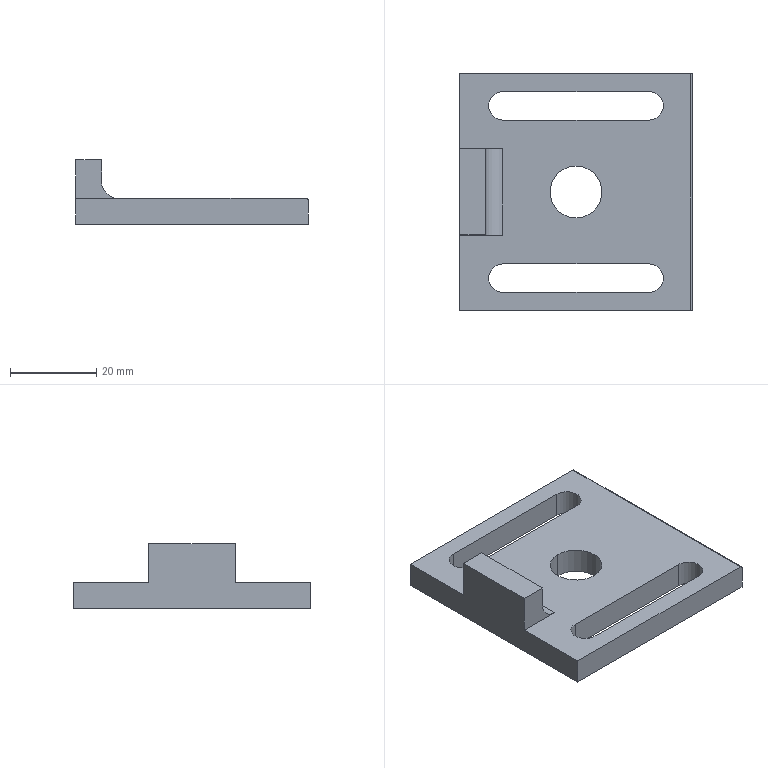Part | STEP file | TNSN20-Y20-F22-Part-4 | 1 solid | 22 faces | box 54 x 55 x 15 mm | volume 15184 mm3 | plane 14 | cylinder 8 | commonest cylinder face diameters 6.6 x4 12 x2 1 x1 8 x1
STEP:
#1=CARTESIAN_POINT('',(14056.745,13710.046,24.));
#2=VERTEX_POINT('',#1);
#3=CARTESIAN_POINT('',(14056.745,13730.046,24.));
#4=VERTEX_POINT('',#3);
#5=CARTESIAN_POINT('',(14056.745,13710.046,24.));
#6=DIRECTION('',(0.,1.,0.));
#7=VECTOR('',#6,1000.);
#8=LINE('',#5,#7);
#9=EDGE_CURVE('',#2,#4,#8,.T.);
#10=ORIENTED_EDGE('',*,*,#9,.T.);
#11=CARTESIAN_POINT('',(14050.745,13730.046,24.));
#12=VERTEX_POINT('',#11);
#13=CARTESIAN_POINT('',(14056.745,13730.046,24.));
#14=DIRECTION('',(-1.,0.,0.));
#15=VECTOR('',#14,1000.);
#16=LINE('',#13,#15);
#17=EDGE_CURVE('',#4,#12,#16,.T.);
#18=ORIENTED_EDGE('',*,*,#17,.T.);
#19=CARTESIAN_POINT('',(14050.745,13710.046,24.));
#20=VERTEX_POINT('',#19);
#21=CARTESIAN_POINT('',(14050.745,13710.046,24.));
#22=DIRECTION('',(0.,1.,0.));
#23=VECTOR('',#22,1000.);
#24=LINE('',#21,#23);
#25=EDGE_CURVE('',#20,#12,#24,.T.);
#26=ORIENTED_EDGE('',*,*,#25,.F.);
#27=CARTESIAN_POINT('',(14050.745,13710.046,24.));
#28=DIRECTION('',(1.,0.,0.));
#29=VECTOR('',#28,1000.);
#30=LINE('',#27,#29);
#31=EDGE_CURVE('',#20,#2,#30,.T.);
#32=ORIENTED_EDGE('',*,*,#31,.T.);
#33=EDGE_LOOP('',(#10,#18,#26,#32));
#34=FACE_OUTER_BOUND('',#33,.T.);
#35=CARTESIAN_POINT('',(14038.084,13704.386,24.));
#36=DIRECTION('',(0.,0.,-1.));
#37=DIRECTION('',(0.,1.,0.));
#38=AXIS2_PLACEMENT_3D('',#35,#36,#37);
#39=PLANE('',#38);
#40=ADVANCED_FACE('',(#34),#39,.F.);
#41=ORIENTED_EDGE('',*,*,#25,.T.);
#42=CARTESIAN_POINT('',(14050.745,13730.046,15.));
#43=VERTEX_POINT('',#42);
#44=CARTESIAN_POINT('',(14050.745,13730.046,24.));
#45=DIRECTION('',(0.,0.,-1.));
#46=VECTOR('',#45,1000.);
#47=LINE('',#44,#46);
#48=EDGE_CURVE('',#12,#43,#47,.T.);
#49=ORIENTED_EDGE('',*,*,#48,.T.);
#50=CARTESIAN_POINT('',(14050.745,13747.546,15.));
#51=VERTEX_POINT('',#50);
#52=CARTESIAN_POINT('',(14050.745,13730.046,15.));
#53=DIRECTION('',(0.,1.,0.));
#54=VECTOR('',#53,1000.);
#55=LINE('',#52,#54);
#56=EDGE_CURVE('',#43,#51,#55,.T.);
#57=ORIENTED_EDGE('',*,*,#56,.T.);
#58=CARTESIAN_POINT('',(14050.745,13747.546,9.));
#59=VERTEX_POINT('',#58);
#60=CARTESIAN_POINT('',(14050.745,13747.546,15.));
#61=DIRECTION('',(0.,0.,-1.));
#62=VECTOR('',#61,1000.);
#63=LINE('',#60,#62);
#64=EDGE_CURVE('',#51,#59,#63,.T.);
#65=ORIENTED_EDGE('',*,*,#64,.T.);
#66=CARTESIAN_POINT('',(14050.745,13692.546,9.));
#67=VERTEX_POINT('',#66);
#68=CARTESIAN_POINT('',(14050.745,13692.546,9.));
#69=DIRECTION('',(0.,1.,0.));
#70=VECTOR('',#69,1000.);
#71=LINE('',#68,#70);
#72=EDGE_CURVE('',#67,#59,#71,.T.);
#73=ORIENTED_EDGE('',*,*,#72,.F.);
#74=CARTESIAN_POINT('',(14050.745,13692.546,15.));
#75=VERTEX_POINT('',#74);
#76=CARTESIAN_POINT('',(14050.745,13692.546,15.));
#77=DIRECTION('',(0.,0.,-1.));
#78=VECTOR('',#77,1000.);
#79=LINE('',#76,#78);
#80=EDGE_CURVE('',#75,#67,#79,.T.);
#81=ORIENTED_EDGE('',*,*,#80,.F.);
#82=CARTESIAN_POINT('',(14050.745,13710.046,15.));
#83=VERTEX_POINT('',#82);
#84=CARTESIAN_POINT('',(14050.745,13692.546,15.));
#85=DIRECTION('',(0.,1.,0.));
#86=VECTOR('',#85,1000.);
#87=LINE('',#84,#86);
#88=EDGE_CURVE('',#75,#83,#87,.T.);
#89=ORIENTED_EDGE('',*,*,#88,.T.);
#90=CARTESIAN_POINT('',(14050.745,13710.046,15.));
#91=DIRECTION('',(0.,0.,1.));
#92=VECTOR('',#91,1000.);
#93=LINE('',#90,#92);
#94=EDGE_CURVE('',#83,#20,#93,.T.);
#95=ORIENTED_EDGE('',*,*,#94,.T.);
#96=EDGE_LOOP('',(#41,#49,#57,#65,#73,#81,#89,#95));
#97=FACE_OUTER_BOUND('',#96,.T.);
#98=CARTESIAN_POINT('',(14050.745,13677.29,-26.257));
#99=DIRECTION('',(1.,0.,0.));
#100=DIRECTION('',(0.,1.,0.));
#101=AXIS2_PLACEMENT_3D('',#98,#99,#100);
#102=PLANE('',#101);
#103=ADVANCED_FACE('',(#97),#102,.F.);
#104=CARTESIAN_POINT('',(14104.745,13747.546,9.));
#105=VERTEX_POINT('',#104);
#106=CARTESIAN_POINT('',(14050.745,13747.546,9.));
#107=DIRECTION('',(1.,0.,0.));
#108=VECTOR('',#107,1000.);
#109=LINE('',#106,#108);
#110=EDGE_CURVE('',#59,#105,#109,.T.);
#111=ORIENTED_EDGE('',*,*,#110,.T.);
#112=CARTESIAN_POINT('',(14104.745,13692.546,9.));
#113=VERTEX_POINT('',#112);
#114=CARTESIAN_POINT('',(14104.745,13692.546,9.));
#115=DIRECTION('',(0.,1.,0.));
#116=VECTOR('',#115,1000.);
#117=LINE('',#114,#116);
#118=EDGE_CURVE('',#113,#105,#117,.T.);
#119=ORIENTED_EDGE('',*,*,#118,.F.);
#120=CARTESIAN_POINT('',(14050.745,13692.546,9.));
#121=DIRECTION('',(1.,0.,0.));
#122=VECTOR('',#121,1000.);
#123=LINE('',#120,#122);
#124=EDGE_CURVE('',#67,#113,#123,.T.);
#125=ORIENTED_EDGE('',*,*,#124,.F.);
#126=ORIENTED_EDGE('',*,*,#72,.T.);
#127=EDGE_LOOP('',(#111,#119,#125,#126));
#128=FACE_OUTER_BOUND('',#127,.T.);
#129=CARTESIAN_POINT('',(14094.745,13703.346,9.));
#130=VERTEX_POINT('',#129);
#131=CARTESIAN_POINT('',(14060.745,13703.346,9.));
#132=VERTEX_POINT('',#131);
#133=CARTESIAN_POINT('',(14094.745,13703.346,9.));
#134=DIRECTION('',(-1.,0.,0.));
#135=VECTOR('',#134,1000.);
#136=LINE('',#133,#135);
#137=EDGE_CURVE('',#130,#132,#136,.T.);
#138=ORIENTED_EDGE('',*,*,#137,.T.);
#139=CARTESIAN_POINT('',(14060.745,13696.746,9.));
#140=VERTEX_POINT('',#139);
#141=CARTESIAN_POINT('',(14060.745,13700.046,9.));
#142=DIRECTION('',(0.,0.,1.));
#143=DIRECTION('',(0.,1.,0.));
#144=AXIS2_PLACEMENT_3D('',#141,#142,#143);
#145=CIRCLE('',#144,3.3);
#146=EDGE_CURVE('',#132,#140,#145,.T.);
#147=ORIENTED_EDGE('',*,*,#146,.T.);
#148=CARTESIAN_POINT('',(14094.745,13696.746,9.));
#149=VERTEX_POINT('',#148);
#150=CARTESIAN_POINT('',(14060.745,13696.746,9.));
#151=DIRECTION('',(1.,0.,0.));
#152=VECTOR('',#151,1000.);
#153=LINE('',#150,#152);
#154=EDGE_CURVE('',#140,#149,#153,.T.);
#155=ORIENTED_EDGE('',*,*,#154,.T.);
#156=CARTESIAN_POINT('',(14094.745,13700.046,9.));
#157=DIRECTION('',(0.,0.,1.));
#158=DIRECTION('',(0.,-1.,0.));
#159=AXIS2_PLACEMENT_3D('',#156,#157,#158);
#160=CIRCLE('',#159,3.3);
#161=EDGE_CURVE('',#149,#130,#160,.T.);
#162=ORIENTED_EDGE('',*,*,#161,.T.);
#163=EDGE_LOOP('',(#138,#147,#155,#162));
#164=FACE_BOUND('',#163,.T.);
#165=CARTESIAN_POINT('',(14094.745,13743.346,9.));
#166=VERTEX_POINT('',#165);
#167=CARTESIAN_POINT('',(14060.745,13743.346,9.));
#168=VERTEX_POINT('',#167);
#169=CARTESIAN_POINT('',(14094.745,13743.346,9.));
#170=DIRECTION('',(-1.,0.,0.));
#171=VECTOR('',#170,1000.);
#172=LINE('',#169,#171);
#173=EDGE_CURVE('',#166,#168,#172,.T.);
#174=ORIENTED_EDGE('',*,*,#173,.T.);
#175=CARTESIAN_POINT('',(14060.745,13736.746,9.));
#176=VERTEX_POINT('',#175);
#177=CARTESIAN_POINT('',(14060.745,13740.046,9.));
#178=DIRECTION('',(0.,0.,1.));
#179=DIRECTION('',(0.,1.,0.));
#180=AXIS2_PLACEMENT_3D('',#177,#178,#179);
#181=CIRCLE('',#180,3.3);
#182=EDGE_CURVE('',#168,#176,#181,.T.);
#183=ORIENTED_EDGE('',*,*,#182,.T.);
#184=CARTESIAN_POINT('',(14094.745,13736.746,9.));
#185=VERTEX_POINT('',#184);
#186=CARTESIAN_POINT('',(14060.745,13736.746,9.));
#187=DIRECTION('',(1.,0.,0.));
#188=VECTOR('',#187,1000.);
#189=LINE('',#186,#188);
#190=EDGE_CURVE('',#176,#185,#189,.T.);
#191=ORIENTED_EDGE('',*,*,#190,.T.);
#192=CARTESIAN_POINT('',(14094.745,13740.046,9.));
#193=DIRECTION('',(0.,0.,1.));
#194=DIRECTION('',(0.,-1.,0.));
#195=AXIS2_PLACEMENT_3D('',#192,#193,#194);
#196=CIRCLE('',#195,3.3);
#197=EDGE_CURVE('',#185,#166,#196,.T.);
#198=ORIENTED_EDGE('',*,*,#197,.T.);
#199=EDGE_LOOP('',(#174,#183,#191,#198));
#200=FACE_BOUND('',#199,.T.);
#201=CARTESIAN_POINT('',(14077.744,13714.046,9.));
#202=VERTEX_POINT('',#201);
#203=CARTESIAN_POINT('',(14077.745,13726.046,9.));
#204=VERTEX_POINT('',#203);
#205=CARTESIAN_POINT('',(14077.745,13720.046,9.));
#206=DIRECTION('',(0.,0.,1.));
#207=DIRECTION('',(1.,0.,0.));
#208=AXIS2_PLACEMENT_3D('',#205,#206,#207);
#209=CIRCLE('',#208,6.);
#210=EDGE_CURVE('',#202,#204,#209,.T.);
#211=ORIENTED_EDGE('',*,*,#210,.T.);
#212=CARTESIAN_POINT('',(14077.745,13720.046,9.));
#213=DIRECTION('',(0.,0.,1.));
#214=DIRECTION('',(1.,0.,0.));
#215=AXIS2_PLACEMENT_3D('',#212,#213,#214);
#216=CIRCLE('',#215,6.);
#217=EDGE_CURVE('',#204,#202,#216,.T.);
#218=ORIENTED_EDGE('',*,*,#217,.T.);
#219=EDGE_LOOP('',(#211,#218));
#220=FACE_BOUND('',#219,.T.);
#221=CARTESIAN_POINT('',(14019.937,13777.855,9.));
#222=DIRECTION('',(0.,0.,1.));
#223=DIRECTION('',(0.,-1.,0.));
#224=AXIS2_PLACEMENT_3D('',#221,#222,#223);
#225=PLANE('',#224);
#226=ADVANCED_FACE('',(#128,#164,#200,#220),#225,.F.);
#227=CARTESIAN_POINT('',(14104.745,13747.546,14.5));
#228=VERTEX_POINT('',#227);
#229=CARTESIAN_POINT('',(14104.745,13747.546,9.));
#230=DIRECTION('',(0.,0.,1.));
#231=VECTOR('',#230,1000.);
#232=LINE('',#229,#231);
#233=EDGE_CURVE('',#105,#228,#232,.T.);
#234=ORIENTED_EDGE('',*,*,#233,.T.);
#235=CARTESIAN_POINT('',(14104.745,13692.546,14.5));
#236=VERTEX_POINT('',#235);
#237=CARTESIAN_POINT('',(14104.745,13692.546,14.5));
#238=DIRECTION('',(0.,1.,0.));
#239=VECTOR('',#238,1000.);
#240=LINE('',#237,#239);
#241=EDGE_CURVE('',#236,#228,#240,.T.);
#242=ORIENTED_EDGE('',*,*,#241,.F.);
#243=CARTESIAN_POINT('',(14104.745,13692.546,9.));
#244=DIRECTION('',(0.,0.,1.));
#245=VECTOR('',#244,1000.);
#246=LINE('',#243,#245);
#247=EDGE_CURVE('',#113,#236,#246,.T.);
#248=ORIENTED_EDGE('',*,*,#247,.F.);
#249=ORIENTED_EDGE('',*,*,#118,.T.);
#250=EDGE_LOOP('',(#234,#242,#248,#249));
#251=FACE_OUTER_BOUND('',#250,.T.);
#252=CARTESIAN_POINT('',(14104.745,13761.502,-29.706));
#253=DIRECTION('',(-1.,0.,0.));
#254=DIRECTION('',(0.,-1.,0.));
#255=AXIS2_PLACEMENT_3D('',#252,#253,#254);
#256=PLANE('',#255);
#257=ADVANCED_FACE('',(#251),#256,.F.);
#258=CARTESIAN_POINT('',(14104.245,13747.546,15.));
#259=VERTEX_POINT('',#258);
#260=CARTESIAN_POINT('',(14104.245,13747.546,14.5));
#261=DIRECTION('',(0.,-1.,0.));
#262=DIRECTION('',(1.,0.,0.));
#263=AXIS2_PLACEMENT_3D('',#260,#261,#262);
#264=CIRCLE('',#263,0.5);
#265=EDGE_CURVE('',#228,#259,#264,.T.);
#266=ORIENTED_EDGE('',*,*,#265,.T.);
#267=CARTESIAN_POINT('',(14104.245,13692.546,15.));
#268=VERTEX_POINT('',#267);
#269=CARTESIAN_POINT('',(14104.245,13692.546,15.));
#270=DIRECTION('',(0.,1.,0.));
#271=VECTOR('',#270,1000.);
#272=LINE('',#269,#271);
#273=EDGE_CURVE('',#268,#259,#272,.T.);
#274=ORIENTED_EDGE('',*,*,#273,.F.);
#275=CARTESIAN_POINT('',(14104.245,13692.546,14.5));
#276=DIRECTION('',(0.,-1.,0.));
#277=DIRECTION('',(1.,0.,0.));
#278=AXIS2_PLACEMENT_3D('',#275,#276,#277);
#279=CIRCLE('',#278,0.5);
#280=EDGE_CURVE('',#236,#268,#279,.T.);
#281=ORIENTED_EDGE('',*,*,#280,.F.);
#282=ORIENTED_EDGE('',*,*,#241,.T.);
#283=EDGE_LOOP('',(#266,#274,#281,#282));
#284=FACE_OUTER_BOUND('',#283,.T.);
#285=CARTESIAN_POINT('',(14104.245,13720.046,14.5));
#286=DIRECTION('',(0.,1.,0.));
#287=DIRECTION('',(-1.,0.,0.));
#288=AXIS2_PLACEMENT_3D('',#285,#286,#287);
#289=CYLINDRICAL_SURFACE('',#288,0.5);
#290=ADVANCED_FACE('',(#284),#289,.T.);
#291=CARTESIAN_POINT('',(14060.745,13730.046,15.));
#292=VERTEX_POINT('',#291);
#293=CARTESIAN_POINT('',(14050.745,13730.046,15.));
#294=DIRECTION('',(1.,0.,0.));
#295=VECTOR('',#294,1000.);
#296=LINE('',#293,#295);
#297=EDGE_CURVE('',#43,#292,#296,.T.);
#298=ORIENTED_EDGE('',*,*,#297,.T.);
#299=CARTESIAN_POINT('',(14060.745,13710.046,15.));
#300=VERTEX_POINT('',#299);
#301=CARTESIAN_POINT('',(14060.745,13710.046,15.));
#302=DIRECTION('',(0.,1.,0.));
#303=VECTOR('',#302,1000.);
#304=LINE('',#301,#303);
#305=EDGE_CURVE('',#300,#292,#304,.T.);
#306=ORIENTED_EDGE('',*,*,#305,.F.);
#307=CARTESIAN_POINT('',(14050.745,13710.046,15.));
#308=DIRECTION('',(1.,0.,0.));
#309=VECTOR('',#308,1000.);
#310=LINE('',#307,#309);
#311=EDGE_CURVE('',#83,#300,#310,.T.);
#312=ORIENTED_EDGE('',*,*,#311,.F.);
#313=ORIENTED_EDGE('',*,*,#88,.F.);
#314=CARTESIAN_POINT('',(14104.245,13692.546,15.));
#315=DIRECTION('',(-1.,0.,0.));
#316=VECTOR('',#315,1000.);
#317=LINE('',#314,#316);
#318=EDGE_CURVE('',#268,#75,#317,.T.);
#319=ORIENTED_EDGE('',*,*,#318,.F.);
#320=ORIENTED_EDGE('',*,*,#273,.T.);
#321=CARTESIAN_POINT('',(14104.245,13747.546,15.));
#322=DIRECTION('',(-1.,0.,0.));
#323=VECTOR('',#322,1000.);
#324=LINE('',#321,#323);
#325=EDGE_CURVE('',#259,#51,#324,.T.);
#326=ORIENTED_EDGE('',*,*,#325,.T.);
#327=ORIENTED_EDGE('',*,*,#56,.F.);
#328=EDGE_LOOP('',(#298,#306,#312,#313,#319,#320,#326,#327));
#329=FACE_OUTER_BOUND('',#328,.T.);
#330=CARTESIAN_POINT('',(14094.745,13703.346,15.));
#331=VERTEX_POINT('',#330);
#332=CARTESIAN_POINT('',(14060.745,13703.346,15.));
#333=VERTEX_POINT('',#332);
#334=CARTESIAN_POINT('',(14094.745,13703.346,15.));
#335=DIRECTION('',(-1.,0.,0.));
#336=VECTOR('',#335,1000.);
#337=LINE('',#334,#336);
#338=EDGE_CURVE('',#331,#333,#337,.T.);
#339=ORIENTED_EDGE('',*,*,#338,.F.);
#340=CARTESIAN_POINT('',(14094.745,13696.746,15.));
#341=VERTEX_POINT('',#340);
#342=CARTESIAN_POINT('',(14094.745,13700.046,15.));
#343=DIRECTION('',(0.,0.,1.));
#344=DIRECTION('',(0.,-1.,0.));
#345=AXIS2_PLACEMENT_3D('',#342,#343,#344);
#346=CIRCLE('',#345,3.3);
#347=EDGE_CURVE('',#341,#331,#346,.T.);
#348=ORIENTED_EDGE('',*,*,#347,.F.);
#349=CARTESIAN_POINT('',(14060.745,13696.746,15.));
#350=VERTEX_POINT('',#349);
#351=CARTESIAN_POINT('',(14060.745,13696.746,15.));
#352=DIRECTION('',(1.,0.,0.));
#353=VECTOR('',#352,1000.);
#354=LINE('',#351,#353);
#355=EDGE_CURVE('',#350,#341,#354,.T.);
#356=ORIENTED_EDGE('',*,*,#355,.F.);
#357=CARTESIAN_POINT('',(14060.745,13700.046,15.));
#358=DIRECTION('',(0.,0.,1.));
#359=DIRECTION('',(0.,1.,0.));
#360=AXIS2_PLACEMENT_3D('',#357,#358,#359);
#361=CIRCLE('',#360,3.3);
#362=EDGE_CURVE('',#333,#350,#361,.T.);
#363=ORIENTED_EDGE('',*,*,#362,.F.);
#364=EDGE_LOOP('',(#339,#348,#356,#363));
#365=FACE_BOUND('',#364,.T.);
#366=CARTESIAN_POINT('',(14094.745,13743.346,15.));
#367=VERTEX_POINT('',#366);
#368=CARTESIAN_POINT('',(14060.745,13743.346,15.));
#369=VERTEX_POINT('',#368);
#370=CARTESIAN_POINT('',(14094.745,13743.346,15.));
#371=DIRECTION('',(-1.,0.,0.));
#372=VECTOR('',#371,1000.);
#373=LINE('',#370,#372);
#374=EDGE_CURVE('',#367,#369,#373,.T.);
#375=ORIENTED_EDGE('',*,*,#374,.F.);
#376=CARTESIAN_POINT('',(14094.745,13736.746,15.));
#377=VERTEX_POINT('',#376);
#378=CARTESIAN_POINT('',(14094.745,13740.046,15.));
#379=DIRECTION('',(0.,0.,1.));
#380=DIRECTION('',(0.,-1.,0.));
#381=AXIS2_PLACEMENT_3D('',#378,#379,#380);
#382=CIRCLE('',#381,3.3);
#383=EDGE_CURVE('',#377,#367,#382,.T.);
#384=ORIENTED_EDGE('',*,*,#383,.F.);
#385=CARTESIAN_POINT('',(14060.745,13736.746,15.));
#386=VERTEX_POINT('',#385);
#387=CARTESIAN_POINT('',(14060.745,13736.746,15.));
#388=DIRECTION('',(1.,0.,0.));
#389=VECTOR('',#388,1000.);
#390=LINE('',#387,#389);
#391=EDGE_CURVE('',#386,#377,#390,.T.);
#392=ORIENTED_EDGE('',*,*,#391,.F.);
#393=CARTESIAN_POINT('',(14060.745,13740.046,15.));
#394=DIRECTION('',(0.,0.,1.));
#395=DIRECTION('',(0.,1.,0.));
#396=AXIS2_PLACEMENT_3D('',#393,#394,#395);
#397=CIRCLE('',#396,3.3);
#398=EDGE_CURVE('',#369,#386,#397,.T.);
#399=ORIENTED_EDGE('',*,*,#398,.F.);
#400=EDGE_LOOP('',(#375,#384,#392,#399));
#401=FACE_BOUND('',#400,.T.);
#402=CARTESIAN_POINT('',(14077.744,13714.046,15.));
#403=VERTEX_POINT('',#402);
#404=CARTESIAN_POINT('',(14077.745,13726.046,15.));
#405=VERTEX_POINT('',#404);
#406=CARTESIAN_POINT('',(14077.745,13720.046,15.));
#407=DIRECTION('',(0.,0.,1.));
#408=DIRECTION('',(1.,0.,0.));
#409=AXIS2_PLACEMENT_3D('',#406,#407,#408);
#410=CIRCLE('',#409,6.);
#411=EDGE_CURVE('',#403,#405,#410,.T.);
#412=ORIENTED_EDGE('',*,*,#411,.F.);
#413=CARTESIAN_POINT('',(14077.745,13720.046,15.));
#414=DIRECTION('',(0.,0.,1.));
#415=DIRECTION('',(1.,0.,0.));
#416=AXIS2_PLACEMENT_3D('',#413,#414,#415);
#417=CIRCLE('',#416,6.);
#418=EDGE_CURVE('',#405,#403,#417,.T.);
#419=ORIENTED_EDGE('',*,*,#418,.F.);
#420=EDGE_LOOP('',(#412,#419));
#421=FACE_BOUND('',#420,.T.);
#422=CARTESIAN_POINT('',(14019.949,13662.5,15.));
#423=DIRECTION('',(0.,0.,-1.));
#424=DIRECTION('',(0.,1.,0.));
#425=AXIS2_PLACEMENT_3D('',#422,#423,#424);
#426=PLANE('',#425);
#427=ADVANCED_FACE('',(#329,#365,#401,#421),#426,.F.);
#428=CARTESIAN_POINT('',(14056.745,13730.046,19.));
#429=VERTEX_POINT('',#428);
#430=CARTESIAN_POINT('',(14060.745,13730.046,19.));
#431=DIRECTION('',(0.,-1.,0.));
#432=DIRECTION('',(-1.,0.,0.));
#433=AXIS2_PLACEMENT_3D('',#430,#431,#432);
#434=CIRCLE('',#433,4.);
#435=EDGE_CURVE('',#429,#292,#434,.T.);
#436=ORIENTED_EDGE('',*,*,#435,.F.);
#437=CARTESIAN_POINT('',(14056.745,13710.046,19.));
#438=VERTEX_POINT('',#437);
#439=CARTESIAN_POINT('',(14056.745,13710.046,19.));
#440=DIRECTION('',(0.,1.,0.));
#441=VECTOR('',#440,1000.);
#442=LINE('',#439,#441);
#443=EDGE_CURVE('',#438,#429,#442,.T.);
#444=ORIENTED_EDGE('',*,*,#443,.F.);
#445=CARTESIAN_POINT('',(14060.745,13710.046,19.));
#446=DIRECTION('',(0.,1.,0.));
#447=DIRECTION('',(0.,0.,-1.));
#448=AXIS2_PLACEMENT_3D('',#445,#446,#447);
#449=CIRCLE('',#448,4.);
#450=EDGE_CURVE('',#300,#438,#449,.T.);
#451=ORIENTED_EDGE('',*,*,#450,.F.);
#452=ORIENTED_EDGE('',*,*,#305,.T.);
#453=EDGE_LOOP('',(#436,#444,#451,#452));
#454=FACE_OUTER_BOUND('',#453,.T.);
#455=CARTESIAN_POINT('',(14060.745,13720.046,19.));
#456=DIRECTION('',(0.,1.,0.));
#457=DIRECTION('',(-1.,0.,0.));
#458=AXIS2_PLACEMENT_3D('',#455,#456,#457);
#459=CYLINDRICAL_SURFACE('',#458,4.);
#460=ADVANCED_FACE('',(#454),#459,.F.);
#461=ORIENTED_EDGE('',*,*,#443,.T.);
#462=CARTESIAN_POINT('',(14056.745,13730.046,19.));
#463=DIRECTION('',(0.,0.,1.));
#464=VECTOR('',#463,1000.);
#465=LINE('',#462,#464);
#466=EDGE_CURVE('',#429,#4,#465,.T.);
#467=ORIENTED_EDGE('',*,*,#466,.T.);
#468=ORIENTED_EDGE('',*,*,#9,.F.);
#469=CARTESIAN_POINT('',(14056.745,13710.046,24.));
#470=DIRECTION('',(0.,0.,-1.));
#471=VECTOR('',#470,1000.);
#472=LINE('',#469,#471);
#473=EDGE_CURVE('',#2,#438,#472,.T.);
#474=ORIENTED_EDGE('',*,*,#473,.T.);
#475=EDGE_LOOP('',(#461,#467,#468,#474));
#476=FACE_OUTER_BOUND('',#475,.T.);
#477=CARTESIAN_POINT('',(14056.745,13735.508,6.038));
#478=DIRECTION('',(-1.,0.,0.));
#479=DIRECTION('',(0.,-1.,0.));
#480=AXIS2_PLACEMENT_3D('',#477,#478,#479);
#481=PLANE('',#480);
#482=ADVANCED_FACE('',(#476),#481,.F.);
#483=ORIENTED_EDGE('',*,*,#318,.T.);
#484=ORIENTED_EDGE('',*,*,#80,.T.);
#485=ORIENTED_EDGE('',*,*,#124,.T.);
#486=ORIENTED_EDGE('',*,*,#247,.T.);
#487=ORIENTED_EDGE('',*,*,#280,.T.);
#488=EDGE_LOOP('',(#483,#484,#485,#486,#487));
#489=FACE_OUTER_BOUND('',#488,.T.);
#490=CARTESIAN_POINT('',(14036.996,13692.546,-28.749));
#491=DIRECTION('',(0.,-1.,0.));
#492=DIRECTION('',(1.,0.,0.));
#493=AXIS2_PLACEMENT_3D('',#490,#491,#492);
#494=PLANE('',#493);
#495=ADVANCED_FACE('',(#489),#494,.T.);
#496=ORIENTED_EDGE('',*,*,#64,.F.);
#497=ORIENTED_EDGE('',*,*,#325,.F.);
#498=ORIENTED_EDGE('',*,*,#265,.F.);
#499=ORIENTED_EDGE('',*,*,#233,.F.);
#500=ORIENTED_EDGE('',*,*,#110,.F.);
#501=EDGE_LOOP('',(#496,#497,#498,#499,#500));
#502=FACE_OUTER_BOUND('',#501,.T.);
#503=CARTESIAN_POINT('',(14036.996,13747.546,-28.749));
#504=DIRECTION('',(0.,-1.,0.));
#505=DIRECTION('',(1.,0.,0.));
#506=AXIS2_PLACEMENT_3D('',#503,#504,#505);
#507=PLANE('',#506);
#508=ADVANCED_FACE('',(#502),#507,.F.);
#509=ORIENTED_EDGE('',*,*,#94,.F.);
#510=ORIENTED_EDGE('',*,*,#311,.T.);
#511=ORIENTED_EDGE('',*,*,#450,.T.);
#512=ORIENTED_EDGE('',*,*,#473,.F.);
#513=ORIENTED_EDGE('',*,*,#31,.F.);
#514=EDGE_LOOP('',(#509,#510,#511,#512,#513));
#515=FACE_OUTER_BOUND('',#514,.T.);
#516=CARTESIAN_POINT('',(14065.835,13710.046,9.41));
#517=DIRECTION('',(0.,1.,0.));
#518=DIRECTION('',(-1.,0.,0.));
#519=AXIS2_PLACEMENT_3D('',#516,#517,#518);
#520=PLANE('',#519);
#521=ADVANCED_FACE('',(#515),#520,.F.);
#522=ORIENTED_EDGE('',*,*,#466,.F.);
#523=ORIENTED_EDGE('',*,*,#435,.T.);
#524=ORIENTED_EDGE('',*,*,#297,.F.);
#525=ORIENTED_EDGE('',*,*,#48,.F.);
#526=ORIENTED_EDGE('',*,*,#17,.F.);
#527=EDGE_LOOP('',(#522,#523,#524,#525,#526));
#528=FACE_OUTER_BOUND('',#527,.T.);
#529=CARTESIAN_POINT('',(14045.655,13730.046,9.41));
#530=DIRECTION('',(0.,-1.,0.));
#531=DIRECTION('',(1.,0.,0.));
#532=AXIS2_PLACEMENT_3D('',#529,#530,#531);
#533=PLANE('',#532);
#534=ADVANCED_FACE('',(#528),#533,.F.);
#535=ORIENTED_EDGE('',*,*,#173,.F.);
#536=CARTESIAN_POINT('',(14094.745,13743.346,15.));
#537=DIRECTION('',(0.,0.,-1.));
#538=VECTOR('',#537,1000.);
#539=LINE('',#536,#538);
#540=EDGE_CURVE('',#367,#166,#539,.T.);
#541=ORIENTED_EDGE('',*,*,#540,.F.);
#542=ORIENTED_EDGE('',*,*,#374,.T.);
#543=CARTESIAN_POINT('',(14060.745,13743.346,15.));
#544=DIRECTION('',(0.,0.,-1.));
#545=VECTOR('',#544,1000.);
#546=LINE('',#543,#545);
#547=EDGE_CURVE('',#369,#168,#546,.T.);
#548=ORIENTED_EDGE('',*,*,#547,.T.);
#549=EDGE_LOOP('',(#535,#541,#542,#548));
#550=FACE_OUTER_BOUND('',#549,.T.);
#551=CARTESIAN_POINT('',(14051.851,13743.346,-13.894));
#552=DIRECTION('',(0.,-1.,0.));
#553=DIRECTION('',(1.,0.,0.));
#554=AXIS2_PLACEMENT_3D('',#551,#552,#553);
#555=PLANE('',#554);
#556=ADVANCED_FACE('',(#550),#555,.T.);
#557=ORIENTED_EDGE('',*,*,#182,.F.);
#558=ORIENTED_EDGE('',*,*,#547,.F.);
#559=ORIENTED_EDGE('',*,*,#398,.T.);
#560=CARTESIAN_POINT('',(14060.745,13736.746,15.));
#561=DIRECTION('',(0.,0.,-1.));
#562=VECTOR('',#561,1000.);
#563=LINE('',#560,#562);
#564=EDGE_CURVE('',#386,#176,#563,.T.);
#565=ORIENTED_EDGE('',*,*,#564,.T.);
#566=EDGE_LOOP('',(#557,#558,#559,#565));
#567=FACE_OUTER_BOUND('',#566,.T.);
#568=CARTESIAN_POINT('',(14060.745,13740.046,12.));
#569=DIRECTION('',(0.,0.,-1.));
#570=DIRECTION('',(0.,1.,0.));
#571=AXIS2_PLACEMENT_3D('',#568,#569,#570);
#572=CYLINDRICAL_SURFACE('',#571,3.3);
#573=ADVANCED_FACE('',(#567),#572,.F.);
#574=ORIENTED_EDGE('',*,*,#190,.F.);
#575=ORIENTED_EDGE('',*,*,#564,.F.);
#576=ORIENTED_EDGE('',*,*,#391,.T.);
#577=CARTESIAN_POINT('',(14094.745,13736.746,15.));
#578=DIRECTION('',(0.,0.,-1.));
#579=VECTOR('',#578,1000.);
#580=LINE('',#577,#579);
#581=EDGE_CURVE('',#377,#185,#580,.T.);
#582=ORIENTED_EDGE('',*,*,#581,.T.);
#583=EDGE_LOOP('',(#574,#575,#576,#582));
#584=FACE_OUTER_BOUND('',#583,.T.);
#585=CARTESIAN_POINT('',(14103.639,13736.746,-13.894));
#586=DIRECTION('',(0.,1.,0.));
#587=DIRECTION('',(-1.,0.,0.));
#588=AXIS2_PLACEMENT_3D('',#585,#586,#587);
#589=PLANE('',#588);
#590=ADVANCED_FACE('',(#584),#589,.T.);
#591=ORIENTED_EDGE('',*,*,#197,.F.);
#592=ORIENTED_EDGE('',*,*,#581,.F.);
#593=ORIENTED_EDGE('',*,*,#383,.T.);
#594=ORIENTED_EDGE('',*,*,#540,.T.);
#595=EDGE_LOOP('',(#591,#592,#593,#594));
#596=FACE_OUTER_BOUND('',#595,.T.);
#597=CARTESIAN_POINT('',(14094.745,13740.046,12.));
#598=DIRECTION('',(0.,0.,-1.));
#599=DIRECTION('',(0.,1.,0.));
#600=AXIS2_PLACEMENT_3D('',#597,#598,#599);
#601=CYLINDRICAL_SURFACE('',#600,3.3);
#602=ADVANCED_FACE('',(#596),#601,.F.);
#603=ORIENTED_EDGE('',*,*,#137,.F.);
#604=CARTESIAN_POINT('',(14094.745,13703.346,15.));
#605=DIRECTION('',(0.,0.,-1.));
#606=VECTOR('',#605,1000.);
#607=LINE('',#604,#606);
#608=EDGE_CURVE('',#331,#130,#607,.T.);
#609=ORIENTED_EDGE('',*,*,#608,.F.);
#610=ORIENTED_EDGE('',*,*,#338,.T.);
#611=CARTESIAN_POINT('',(14060.745,13703.346,15.));
#612=DIRECTION('',(0.,0.,-1.));
#613=VECTOR('',#612,1000.);
#614=LINE('',#611,#613);
#615=EDGE_CURVE('',#333,#132,#614,.T.);
#616=ORIENTED_EDGE('',*,*,#615,.T.);
#617=EDGE_LOOP('',(#603,#609,#610,#616));
#618=FACE_OUTER_BOUND('',#617,.T.);
#619=CARTESIAN_POINT('',(14051.851,13703.346,-13.894));
#620=DIRECTION('',(0.,-1.,0.));
#621=DIRECTION('',(1.,0.,0.));
#622=AXIS2_PLACEMENT_3D('',#619,#620,#621);
#623=PLANE('',#622);
#624=ADVANCED_FACE('',(#618),#623,.T.);
#625=ORIENTED_EDGE('',*,*,#146,.F.);
#626=ORIENTED_EDGE('',*,*,#615,.F.);
#627=ORIENTED_EDGE('',*,*,#362,.T.);
#628=CARTESIAN_POINT('',(14060.745,13696.746,15.));
#629=DIRECTION('',(0.,0.,-1.));
#630=VECTOR('',#629,1000.);
#631=LINE('',#628,#630);
#632=EDGE_CURVE('',#350,#140,#631,.T.);
#633=ORIENTED_EDGE('',*,*,#632,.T.);
#634=EDGE_LOOP('',(#625,#626,#627,#633));
#635=FACE_OUTER_BOUND('',#634,.T.);
#636=CARTESIAN_POINT('',(14060.745,13700.046,12.));
#637=DIRECTION('',(0.,0.,-1.));
#638=DIRECTION('',(0.,1.,0.));
#639=AXIS2_PLACEMENT_3D('',#636,#637,#638);
#640=CYLINDRICAL_SURFACE('',#639,3.3);
#641=ADVANCED_FACE('',(#635),#640,.F.);
#642=ORIENTED_EDGE('',*,*,#154,.F.);
#643=ORIENTED_EDGE('',*,*,#632,.F.);
#644=ORIENTED_EDGE('',*,*,#355,.T.);
#645=CARTESIAN_POINT('',(14094.745,13696.746,15.));
#646=DIRECTION('',(0.,0.,-1.));
#647=VECTOR('',#646,1000.);
#648=LINE('',#645,#647);
#649=EDGE_CURVE('',#341,#149,#648,.T.);
#650=ORIENTED_EDGE('',*,*,#649,.T.);
#651=EDGE_LOOP('',(#642,#643,#644,#650));
#652=FACE_OUTER_BOUND('',#651,.T.);
#653=CARTESIAN_POINT('',(14103.639,13696.746,-13.894));
#654=DIRECTION('',(0.,1.,0.));
#655=DIRECTION('',(-1.,0.,0.));
#656=AXIS2_PLACEMENT_3D('',#653,#654,#655);
#657=PLANE('',#656);
#658=ADVANCED_FACE('',(#652),#657,.T.);
#659=ORIENTED_EDGE('',*,*,#161,.F.);
#660=ORIENTED_EDGE('',*,*,#649,.F.);
#661=ORIENTED_EDGE('',*,*,#347,.T.);
#662=ORIENTED_EDGE('',*,*,#608,.T.);
#663=EDGE_LOOP('',(#659,#660,#661,#662));
#664=FACE_OUTER_BOUND('',#663,.T.);
#665=CARTESIAN_POINT('',(14094.745,13700.046,12.));
#666=DIRECTION('',(0.,0.,-1.));
#667=DIRECTION('',(0.,1.,0.));
#668=AXIS2_PLACEMENT_3D('',#665,#666,#667);
#669=CYLINDRICAL_SURFACE('',#668,3.3);
#670=ADVANCED_FACE('',(#664),#669,.F.);
#671=CARTESIAN_POINT('',(14077.745,13714.046,15.));
#672=DIRECTION('',(0.,0.,-1.));
#673=VECTOR('',#672,1000.);
#674=LINE('',#671,#673);
#675=EDGE_CURVE('',#403,#202,#674,.T.);
#676=ORIENTED_EDGE('',*,*,#675,.F.);
#677=ORIENTED_EDGE('',*,*,#411,.T.);
#678=CARTESIAN_POINT('',(14077.745,13726.046,15.));
#679=DIRECTION('',(0.,0.,-1.));
#680=VECTOR('',#679,1000.);
#681=LINE('',#678,#680);
#682=EDGE_CURVE('',#405,#204,#681,.T.);
#683=ORIENTED_EDGE('',*,*,#682,.T.);
#684=ORIENTED_EDGE('',*,*,#210,.F.);
#685=EDGE_LOOP('',(#676,#677,#683,#684));
#686=FACE_OUTER_BOUND('',#685,.T.);
#687=CARTESIAN_POINT('',(14077.745,13720.046,12.));
#688=DIRECTION('',(0.,0.,-1.));
#689=DIRECTION('',(0.,1.,0.));
#690=AXIS2_PLACEMENT_3D('',#687,#688,#689);
#691=CYLINDRICAL_SURFACE('',#690,6.);
#692=ADVANCED_FACE('',(#686),#691,.F.);
#693=ORIENTED_EDGE('',*,*,#217,.F.);
#694=ORIENTED_EDGE('',*,*,#682,.F.);
#695=ORIENTED_EDGE('',*,*,#418,.T.);
#696=ORIENTED_EDGE('',*,*,#675,.T.);
#697=EDGE_LOOP('',(#693,#694,#695,#696));
#698=FACE_OUTER_BOUND('',#697,.T.);
#699=CARTESIAN_POINT('',(14077.745,13720.046,12.));
#700=DIRECTION('',(0.,0.,-1.));
#701=DIRECTION('',(0.,1.,0.));
#702=AXIS2_PLACEMENT_3D('',#699,#700,#701);
#703=CYLINDRICAL_SURFACE('',#702,6.);
#704=ADVANCED_FACE('',(#698),#703,.F.);
#705=CLOSED_SHELL('',(#40,#103,#226,#257,#290,#427,#460,#482,#495,#508,#521,#534,#556,#573,#590,#602,#624,#641,#658,#670,#692,#704));
#706=MANIFOLD_SOLID_BREP('',#705);
#707=CARTESIAN_POINT('',(0.,0.,0.));
#708=DIRECTION('',(0.,0.,1.));
#709=DIRECTION('',(1.,0.,0.));
#710=AXIS2_PLACEMENT_3D('',#707,#708,#709);
#711=(LENGTH_UNIT()NAMED_UNIT(*)SI_UNIT(.MILLI.,.METRE.));
#712=UNCERTAINTY_MEASURE_WITH_UNIT(LENGTH_MEASURE(0.00001),#711,'','');
#713=(NAMED_UNIT(*)PLANE_ANGLE_UNIT()SI_UNIT($,.RADIAN.));
#714=(NAMED_UNIT(*)SI_UNIT($,.STERADIAN.)SOLID_ANGLE_UNIT());
#715=(GEOMETRIC_REPRESENTATION_CONTEXT(3)GLOBAL_UNCERTAINTY_ASSIGNED_CONTEXT((#712))GLOBAL_UNIT_ASSIGNED_CONTEXT((#711,#713,#714))REPRESENTATION_CONTEXT('',''));
#716=ADVANCED_BREP_SHAPE_REPRESENTATION('',(#706,#710),#715);